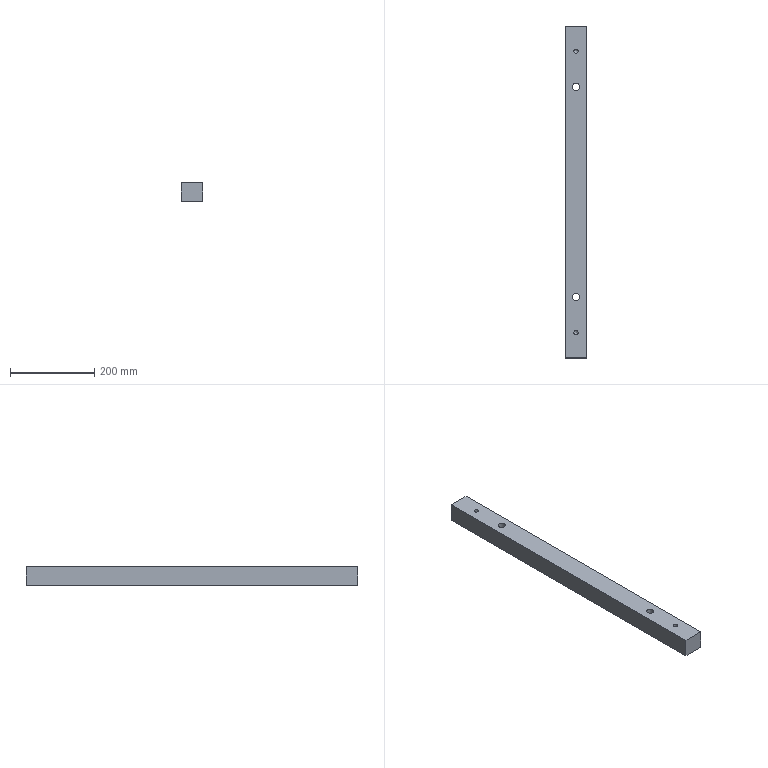Part | STEP file | 014_id2198_x_t | 1 solid | 16 faces | box 50 x 790 x 45 mm | volume 1744458 mm3 | plane 6 | cylinder 6 | cone 4 | commonest cylinder face diameters 10.3 x2 14 x2 17 x2
STEP:
#1=CARTESIAN_POINT('',(0.,0.,0.));
#2=DIRECTION('',(0.,0.,1.));
#3=DIRECTION('',(1.,0.,0.));
#4=AXIS2_PLACEMENT_3D('',#1,#2,#3);
#5=CARTESIAN_POINT('',(-521.65,-335.,230.));
#6=VERTEX_POINT('',#5);
#7=CARTESIAN_POINT('',(-516.5,-335.,230.));
#8=DIRECTION('',(0.,0.,-1.));
#9=DIRECTION('',(-1.,0.,0.));
#10=AXIS2_PLACEMENT_3D('',#7,#8,#9);
#11=CIRCLE('',#10,5.15);
#12=CARTESIAN_POINT('',(-541.5,-250.,230.));
#13=DIRECTION('',(0.,0.,-1.));
#14=DIRECTION('',(0.,-1.,0.));
#15=AXIS2_PLACEMENT_3D('',#12,#13,#14);
#16=PLANE('',#15);
#17=CARTESIAN_POINT('',(85.,-25.));
#18=DIRECTION('',(0.,1.));
#19=AXIS2_PLACEMENT_2D('',#17,#18);
#20=CIRCLE('',#19,5.15);
#21=(GEOMETRIC_REPRESENTATION_CONTEXT(2)PARAMETRIC_REPRESENTATION_CONTEXT()REPRESENTATION_CONTEXT('',''));
#22=DEFINITIONAL_REPRESENTATION('',(#20),#21);
#23=PCURVE('',#16,#22);
#24=CARTESIAN_POINT('',(-516.5,-335.,259.));
#25=DIRECTION('',(0.,0.,-1.));
#26=DIRECTION('',(-1.,0.,0.));
#27=AXIS2_PLACEMENT_3D('',#24,#25,#26);
#28=CYLINDRICAL_SURFACE('',#27,5.15);
#29=CARTESIAN_POINT('',(0.,29.));
#30=DIRECTION('',(1.,0.));
#31=VECTOR('',#30,1.);
#32=LINE('',#29,#31);
#33=(GEOMETRIC_REPRESENTATION_CONTEXT(2)PARAMETRIC_REPRESENTATION_CONTEXT()REPRESENTATION_CONTEXT('',''));
#34=DEFINITIONAL_REPRESENTATION('',(#32),#33);
#35=PCURVE('',#28,#34);
#36=SURFACE_CURVE('',#11,(#23,#35),.PCURVE_S1.);
#37=EDGE_CURVE('',#6,#6,#36,.T.);
#38=ORIENTED_EDGE('',*,*,#37,.T.);
#39=EDGE_LOOP('',(#38));
#40=FACE_BOUND('',#39,.T.);
#41=CARTESIAN_POINT('',(-521.65,335.,230.));
#42=VERTEX_POINT('',#41);
#43=CARTESIAN_POINT('',(-516.5,335.,230.));
#44=DIRECTION('',(0.,0.,1.));
#45=DIRECTION('',(-1.,0.,0.));
#46=AXIS2_PLACEMENT_3D('',#43,#44,#45);
#47=CIRCLE('',#46,5.15);
#48=CARTESIAN_POINT('',(-585.,-19.85));
#49=CARTESIAN_POINT('',(-576.08,-19.85));
#50=CARTESIAN_POINT('',(-580.54,-27.575));
#51=CARTESIAN_POINT('',(-585.,-35.3));
#52=CARTESIAN_POINT('',(-589.46,-27.575));
#53=CARTESIAN_POINT('',(-593.92,-19.85));
#54=CARTESIAN_POINT('',(-585.,-19.85));
#55=(BOUNDED_CURVE()B_SPLINE_CURVE(2,(#48,#49,#50,#51,#52,#53,#54),.UNSPECIFIED.,.T.,.F.)B_SPLINE_CURVE_WITH_KNOTS((1,2,2,2,2,1),(-2.094,0.,2.094,4.189,6.283,8.378),.UNSPECIFIED.)CURVE()GEOMETRIC_REPRESENTATION_ITEM()RATIONAL_B_SPLINE_CURVE((1.,0.5,1.,0.5,1.,0.5,1.))REPRESENTATION_ITEM(''));
#56=(GEOMETRIC_REPRESENTATION_CONTEXT(2)PARAMETRIC_REPRESENTATION_CONTEXT()REPRESENTATION_CONTEXT('',''));
#57=DEFINITIONAL_REPRESENTATION('',(#55),#56);
#58=PCURVE('',#16,#57);
#59=CARTESIAN_POINT('',(-516.5,335.,259.));
#60=DIRECTION('',(0.,0.,-1.));
#61=DIRECTION('',(-1.,0.,0.));
#62=AXIS2_PLACEMENT_3D('',#59,#60,#61);
#63=CYLINDRICAL_SURFACE('',#62,5.15);
#64=CARTESIAN_POINT('',(6.283,29.));
#65=DIRECTION('',(-1.,0.));
#66=VECTOR('',#65,1.);
#67=LINE('',#64,#66);
#68=(GEOMETRIC_REPRESENTATION_CONTEXT(2)PARAMETRIC_REPRESENTATION_CONTEXT()REPRESENTATION_CONTEXT('',''));
#69=DEFINITIONAL_REPRESENTATION('',(#67),#68);
#70=PCURVE('',#63,#69);
#71=SURFACE_CURVE('',#47,(#58,#70),.PCURVE_S1.);
#72=EDGE_CURVE('',#42,#42,#71,.T.);
#73=ORIENTED_EDGE('',*,*,#72,.F.);
#74=EDGE_LOOP('',(#73));
#75=FACE_BOUND('',#74,.T.);
#76=CARTESIAN_POINT('',(-541.5,-395.,230.));
#77=VERTEX_POINT('',#76);
#78=CARTESIAN_POINT('',(-491.5,-395.,230.));
#79=VERTEX_POINT('',#78);
#80=CARTESIAN_POINT('',(-541.5,-395.,230.));
#81=DIRECTION('',(1.,0.,0.));
#82=VECTOR('',#81,1.);
#83=LINE('',#80,#82);
#84=CARTESIAN_POINT('',(145.,0.));
#85=DIRECTION('',(0.,-1.));
#86=VECTOR('',#85,1.);
#87=LINE('',#84,#86);
#88=(GEOMETRIC_REPRESENTATION_CONTEXT(2)PARAMETRIC_REPRESENTATION_CONTEXT()REPRESENTATION_CONTEXT('',''));
#89=DEFINITIONAL_REPRESENTATION('',(#87),#88);
#90=PCURVE('',#16,#89);
#91=CARTESIAN_POINT('',(-541.5,-395.,-28.5));
#92=DIRECTION('',(0.,1.,0.));
#93=DIRECTION('',(0.,0.,-1.));
#94=AXIS2_PLACEMENT_3D('',#91,#92,#93);
#95=PLANE('',#94);
#96=CARTESIAN_POINT('',(-258.5,0.));
#97=DIRECTION('',(0.,-1.));
#98=VECTOR('',#97,1.);
#99=LINE('',#96,#98);
#100=(GEOMETRIC_REPRESENTATION_CONTEXT(2)PARAMETRIC_REPRESENTATION_CONTEXT()REPRESENTATION_CONTEXT('',''));
#101=DEFINITIONAL_REPRESENTATION('',(#99),#100);
#102=PCURVE('',#95,#101);
#103=SURFACE_CURVE('',#83,(#90,#102),.PCURVE_S1.);
#104=EDGE_CURVE('',#77,#79,#103,.T.);
#105=ORIENTED_EDGE('',*,*,#104,.T.);
#106=CARTESIAN_POINT('',(-491.5,395.,230.));
#107=VERTEX_POINT('',#106);
#108=CARTESIAN_POINT('',(-491.5,-250.,230.));
#109=DIRECTION('',(0.,-1.,0.));
#110=VECTOR('',#109,1.);
#111=LINE('',#108,#110);
#112=CARTESIAN_POINT('',(0.,-50.));
#113=DIRECTION('',(1.,0.));
#114=VECTOR('',#113,1.);
#115=LINE('',#112,#114);
#116=(GEOMETRIC_REPRESENTATION_CONTEXT(2)PARAMETRIC_REPRESENTATION_CONTEXT()REPRESENTATION_CONTEXT('',''));
#117=DEFINITIONAL_REPRESENTATION('',(#115),#116);
#118=PCURVE('',#16,#117);
#119=CARTESIAN_POINT('',(-491.5,-250.,-28.5));
#120=DIRECTION('',(-1.,0.,0.));
#121=DIRECTION('',(0.,0.,1.));
#122=AXIS2_PLACEMENT_3D('',#119,#120,#121);
#123=PLANE('',#122);
#124=CARTESIAN_POINT('',(258.5,0.));
#125=DIRECTION('',(0.,-1.));
#126=VECTOR('',#125,1.);
#127=LINE('',#124,#126);
#128=(GEOMETRIC_REPRESENTATION_CONTEXT(2)PARAMETRIC_REPRESENTATION_CONTEXT()REPRESENTATION_CONTEXT('',''));
#129=DEFINITIONAL_REPRESENTATION('',(#127),#128);
#130=PCURVE('',#123,#129);
#131=SURFACE_CURVE('',#111,(#118,#130),.PCURVE_S1.);
#132=EDGE_CURVE('',#107,#79,#131,.T.);
#133=ORIENTED_EDGE('',*,*,#132,.F.);
#134=CARTESIAN_POINT('',(-541.5,395.,230.));
#135=VERTEX_POINT('',#134);
#136=CARTESIAN_POINT('',(-541.5,395.,230.));
#137=DIRECTION('',(1.,0.,0.));
#138=VECTOR('',#137,1.);
#139=LINE('',#136,#138);
#140=CARTESIAN_POINT('',(-645.,0.));
#141=DIRECTION('',(0.,-1.));
#142=VECTOR('',#141,1.);
#143=LINE('',#140,#142);
#144=(GEOMETRIC_REPRESENTATION_CONTEXT(2)PARAMETRIC_REPRESENTATION_CONTEXT()REPRESENTATION_CONTEXT('',''));
#145=DEFINITIONAL_REPRESENTATION('',(#143),#144);
#146=PCURVE('',#16,#145);
#147=CARTESIAN_POINT('',(-541.5,395.,-28.5));
#148=DIRECTION('',(0.,1.,0.));
#149=DIRECTION('',(0.,0.,-1.));
#150=AXIS2_PLACEMENT_3D('',#147,#148,#149);
#151=PLANE('',#150);
#152=CARTESIAN_POINT('',(-258.5,0.));
#153=DIRECTION('',(0.,-1.));
#154=VECTOR('',#153,1.);
#155=LINE('',#152,#154);
#156=(GEOMETRIC_REPRESENTATION_CONTEXT(2)PARAMETRIC_REPRESENTATION_CONTEXT()REPRESENTATION_CONTEXT('',''));
#157=DEFINITIONAL_REPRESENTATION('',(#155),#156);
#158=PCURVE('',#151,#157);
#159=SURFACE_CURVE('',#139,(#146,#158),.PCURVE_S1.);
#160=EDGE_CURVE('',#135,#107,#159,.T.);
#161=ORIENTED_EDGE('',*,*,#160,.F.);
#162=CARTESIAN_POINT('',(-541.5,-250.,230.));
#163=DIRECTION('',(0.,-1.,0.));
#164=VECTOR('',#163,1.);
#165=LINE('',#162,#164);
#166=CARTESIAN_POINT('',(0.,0.));
#167=DIRECTION('',(1.,0.));
#168=VECTOR('',#167,1.);
#169=LINE('',#166,#168);
#170=(GEOMETRIC_REPRESENTATION_CONTEXT(2)PARAMETRIC_REPRESENTATION_CONTEXT()REPRESENTATION_CONTEXT('',''));
#171=DEFINITIONAL_REPRESENTATION('',(#169),#170);
#172=PCURVE('',#16,#171);
#173=CARTESIAN_POINT('',(-541.5,-250.,-28.5));
#174=DIRECTION('',(-1.,0.,0.));
#175=DIRECTION('',(0.,0.,1.));
#176=AXIS2_PLACEMENT_3D('',#173,#174,#175);
#177=PLANE('',#176);
#178=CARTESIAN_POINT('',(258.5,0.));
#179=DIRECTION('',(0.,-1.));
#180=VECTOR('',#179,1.);
#181=LINE('',#178,#180);
#182=(GEOMETRIC_REPRESENTATION_CONTEXT(2)PARAMETRIC_REPRESENTATION_CONTEXT()REPRESENTATION_CONTEXT('',''));
#183=DEFINITIONAL_REPRESENTATION('',(#181),#182);
#184=PCURVE('',#177,#183);
#185=SURFACE_CURVE('',#165,(#172,#184),.PCURVE_S1.);
#186=EDGE_CURVE('',#135,#77,#185,.T.);
#187=ORIENTED_EDGE('',*,*,#186,.T.);
#188=EDGE_LOOP('',(#105,#133,#161,#187));
#189=FACE_BOUND('',#188,.T.);
#190=CARTESIAN_POINT('',(-525.,250.,230.));
#191=VERTEX_POINT('',#190);
#192=CARTESIAN_POINT('',(-516.5,250.,230.));
#193=DIRECTION('',(0.,0.,-1.));
#194=DIRECTION('',(-1.,0.,0.));
#195=AXIS2_PLACEMENT_3D('',#192,#193,#194);
#196=CIRCLE('',#195,8.5);
#197=CARTESIAN_POINT('',(-500.,-25.));
#198=DIRECTION('',(0.,1.));
#199=AXIS2_PLACEMENT_2D('',#197,#198);
#200=CIRCLE('',#199,8.5);
#201=(GEOMETRIC_REPRESENTATION_CONTEXT(2)PARAMETRIC_REPRESENTATION_CONTEXT()REPRESENTATION_CONTEXT('',''));
#202=DEFINITIONAL_REPRESENTATION('',(#200),#201);
#203=PCURVE('',#16,#202);
#204=CARTESIAN_POINT('',(-516.5,250.,150.016));
#205=DIRECTION('',(0.,0.,1.));
#206=DIRECTION('',(1.,0.,0.));
#207=AXIS2_PLACEMENT_3D('',#204,#205,#206);
#208=CYLINDRICAL_SURFACE('',#207,8.5);
#209=CARTESIAN_POINT('',(9.425,79.984));
#210=DIRECTION('',(-1.,0.));
#211=VECTOR('',#210,1.);
#212=LINE('',#209,#211);
#213=(GEOMETRIC_REPRESENTATION_CONTEXT(2)PARAMETRIC_REPRESENTATION_CONTEXT()REPRESENTATION_CONTEXT('',''));
#214=DEFINITIONAL_REPRESENTATION('',(#212),#213);
#215=PCURVE('',#208,#214);
#216=SURFACE_CURVE('',#196,(#203,#215),.PCURVE_S1.);
#217=EDGE_CURVE('',#191,#191,#216,.T.);
#218=ORIENTED_EDGE('',*,*,#217,.T.);
#219=EDGE_LOOP('',(#218));
#220=FACE_BOUND('',#219,.T.);
#221=CARTESIAN_POINT('',(-525.,-250.,230.));
#222=VERTEX_POINT('',#221);
#223=CARTESIAN_POINT('',(-516.5,-250.,230.));
#224=DIRECTION('',(0.,0.,-1.));
#225=DIRECTION('',(-1.,0.,0.));
#226=AXIS2_PLACEMENT_3D('',#223,#224,#225);
#227=CIRCLE('',#226,8.5);
#228=CARTESIAN_POINT('',(0.,-25.));
#229=DIRECTION('',(0.,1.));
#230=AXIS2_PLACEMENT_2D('',#228,#229);
#231=CIRCLE('',#230,8.5);
#232=(GEOMETRIC_REPRESENTATION_CONTEXT(2)PARAMETRIC_REPRESENTATION_CONTEXT()REPRESENTATION_CONTEXT('',''));
#233=DEFINITIONAL_REPRESENTATION('',(#231),#232);
#234=PCURVE('',#16,#233);
#235=CARTESIAN_POINT('',(-516.5,-250.,150.016));
#236=DIRECTION('',(0.,0.,1.));
#237=DIRECTION('',(1.,0.,0.));
#238=AXIS2_PLACEMENT_3D('',#235,#236,#237);
#239=CYLINDRICAL_SURFACE('',#238,8.5);
#240=CARTESIAN_POINT('',(9.425,79.984));
#241=DIRECTION('',(-1.,0.));
#242=VECTOR('',#241,1.);
#243=LINE('',#240,#242);
#244=(GEOMETRIC_REPRESENTATION_CONTEXT(2)PARAMETRIC_REPRESENTATION_CONTEXT()REPRESENTATION_CONTEXT('',''));
#245=DEFINITIONAL_REPRESENTATION('',(#243),#244);
#246=PCURVE('',#239,#245);
#247=SURFACE_CURVE('',#227,(#234,#246),.PCURVE_S1.);
#248=EDGE_CURVE('',#222,#222,#247,.T.);
#249=ORIENTED_EDGE('',*,*,#248,.T.);
#250=EDGE_LOOP('',(#249));
#251=FACE_BOUND('',#250,.T.);
#252=ADVANCED_FACE('',(#40,#75,#189,#220,#251),#16,.F.);
#253=CARTESIAN_POINT('',(-525.,-250.,185.));
#254=VERTEX_POINT('',#253);
#255=CARTESIAN_POINT('',(-516.5,-250.,185.));
#256=DIRECTION('',(0.,0.,-1.));
#257=DIRECTION('',(-1.,0.,0.));
#258=AXIS2_PLACEMENT_3D('',#255,#256,#257);
#259=CIRCLE('',#258,8.5);
#260=CARTESIAN_POINT('',(-336.5,-40.,185.));
#261=DIRECTION('',(0.,0.,-1.));
#262=DIRECTION('',(1.,0.,0.));
#263=AXIS2_PLACEMENT_3D('',#260,#261,#262);
#264=PLANE('',#263);
#265=CARTESIAN_POINT('',(-180.,210.));
#266=DIRECTION('',(-1.,0.));
#267=AXIS2_PLACEMENT_2D('',#265,#266);
#268=CIRCLE('',#267,8.5);
#269=(GEOMETRIC_REPRESENTATION_CONTEXT(2)PARAMETRIC_REPRESENTATION_CONTEXT()REPRESENTATION_CONTEXT('',''));
#270=DEFINITIONAL_REPRESENTATION('',(#268),#269);
#271=PCURVE('',#264,#270);
#272=CARTESIAN_POINT('',(9.425,34.984));
#273=DIRECTION('',(-1.,0.));
#274=VECTOR('',#273,1.);
#275=LINE('',#272,#274);
#276=(GEOMETRIC_REPRESENTATION_CONTEXT(2)PARAMETRIC_REPRESENTATION_CONTEXT()REPRESENTATION_CONTEXT('',''));
#277=DEFINITIONAL_REPRESENTATION('',(#275),#276);
#278=PCURVE('',#239,#277);
#279=SURFACE_CURVE('',#259,(#271,#278),.PCURVE_S1.);
#280=EDGE_CURVE('',#254,#254,#279,.T.);
#281=ORIENTED_EDGE('',*,*,#280,.F.);
#282=EDGE_LOOP('',(#281));
#283=FACE_BOUND('',#282,.T.);
#284=CARTESIAN_POINT('',(-525.,250.,185.));
#285=VERTEX_POINT('',#284);
#286=CARTESIAN_POINT('',(-516.5,250.,185.));
#287=DIRECTION('',(0.,0.,-1.));
#288=DIRECTION('',(-1.,0.,0.));
#289=AXIS2_PLACEMENT_3D('',#286,#287,#288);
#290=CIRCLE('',#289,8.5);
#291=CARTESIAN_POINT('',(-180.,-290.));
#292=DIRECTION('',(-1.,0.));
#293=AXIS2_PLACEMENT_2D('',#291,#292);
#294=CIRCLE('',#293,8.5);
#295=(GEOMETRIC_REPRESENTATION_CONTEXT(2)PARAMETRIC_REPRESENTATION_CONTEXT()REPRESENTATION_CONTEXT('',''));
#296=DEFINITIONAL_REPRESENTATION('',(#294),#295);
#297=PCURVE('',#264,#296);
#298=CARTESIAN_POINT('',(9.425,34.984));
#299=DIRECTION('',(-1.,0.));
#300=VECTOR('',#299,1.);
#301=LINE('',#298,#300);
#302=(GEOMETRIC_REPRESENTATION_CONTEXT(2)PARAMETRIC_REPRESENTATION_CONTEXT()REPRESENTATION_CONTEXT('',''));
#303=DEFINITIONAL_REPRESENTATION('',(#301),#302);
#304=PCURVE('',#208,#303);
#305=SURFACE_CURVE('',#290,(#297,#304),.PCURVE_S1.);
#306=EDGE_CURVE('',#285,#285,#305,.T.);
#307=ORIENTED_EDGE('',*,*,#306,.F.);
#308=EDGE_LOOP('',(#307));
#309=FACE_BOUND('',#308,.T.);
#310=CARTESIAN_POINT('',(-523.5,-370.,185.));
#311=VERTEX_POINT('',#310);
#312=CARTESIAN_POINT('',(-516.5,-370.,185.));
#313=DIRECTION('',(0.,0.,-1.));
#314=DIRECTION('',(-1.,0.,0.));
#315=AXIS2_PLACEMENT_3D('',#312,#313,#314);
#316=CIRCLE('',#315,7.);
#317=CARTESIAN_POINT('',(-180.,330.));
#318=DIRECTION('',(-1.,0.));
#319=AXIS2_PLACEMENT_2D('',#317,#318);
#320=CIRCLE('',#319,7.);
#321=(GEOMETRIC_REPRESENTATION_CONTEXT(2)PARAMETRIC_REPRESENTATION_CONTEXT()REPRESENTATION_CONTEXT('',''));
#322=DEFINITIONAL_REPRESENTATION('',(#320),#321);
#323=PCURVE('',#264,#322);
#324=CARTESIAN_POINT('',(-516.5,-370.,121.));
#325=DIRECTION('',(0.,0.,1.));
#326=DIRECTION('',(1.,0.,0.));
#327=AXIS2_PLACEMENT_3D('',#324,#325,#326);
#328=CYLINDRICAL_SURFACE('',#327,7.);
#329=CARTESIAN_POINT('',(9.425,64.));
#330=DIRECTION('',(-1.,0.));
#331=VECTOR('',#330,1.);
#332=LINE('',#329,#331);
#333=(GEOMETRIC_REPRESENTATION_CONTEXT(2)PARAMETRIC_REPRESENTATION_CONTEXT()REPRESENTATION_CONTEXT('',''));
#334=DEFINITIONAL_REPRESENTATION('',(#332),#333);
#335=PCURVE('',#328,#334);
#336=SURFACE_CURVE('',#316,(#323,#335),.PCURVE_S1.);
#337=EDGE_CURVE('',#311,#311,#336,.T.);
#338=ORIENTED_EDGE('',*,*,#337,.F.);
#339=EDGE_LOOP('',(#338));
#340=FACE_BOUND('',#339,.T.);
#341=CARTESIAN_POINT('',(-523.5,370.,185.));
#342=VERTEX_POINT('',#341);
#343=CARTESIAN_POINT('',(-509.5,370.,185.));
#344=VERTEX_POINT('',#343);
#345=CARTESIAN_POINT('',(-516.5,370.,185.));
#346=DIRECTION('',(0.,0.,-1.));
#347=DIRECTION('',(-1.,0.,0.));
#348=AXIS2_PLACEMENT_3D('',#345,#346,#347);
#349=CIRCLE('',#348,7.);
#350=CARTESIAN_POINT('',(-180.,-410.));
#351=DIRECTION('',(-1.,0.));
#352=AXIS2_PLACEMENT_2D('',#350,#351);
#353=CIRCLE('',#352,7.);
#354=(GEOMETRIC_REPRESENTATION_CONTEXT(2)PARAMETRIC_REPRESENTATION_CONTEXT()REPRESENTATION_CONTEXT('',''));
#355=DEFINITIONAL_REPRESENTATION('',(#353),#354);
#356=PCURVE('',#264,#355);
#357=CARTESIAN_POINT('',(-516.5,370.,121.));
#358=DIRECTION('',(0.,0.,1.));
#359=DIRECTION('',(1.,0.,0.));
#360=AXIS2_PLACEMENT_3D('',#357,#358,#359);
#361=CYLINDRICAL_SURFACE('',#360,7.);
#362=CARTESIAN_POINT('',(3.142,64.));
#363=DIRECTION('',(-1.,0.));
#364=VECTOR('',#363,1.);
#365=LINE('',#362,#364);
#366=(GEOMETRIC_REPRESENTATION_CONTEXT(2)PARAMETRIC_REPRESENTATION_CONTEXT()REPRESENTATION_CONTEXT('',''));
#367=DEFINITIONAL_REPRESENTATION('',(#365),#366);
#368=PCURVE('',#361,#367);
#369=SURFACE_CURVE('',#349,(#356,#368),.PCURVE_S1.);
#370=EDGE_CURVE('',#342,#344,#369,.T.);
#371=ORIENTED_EDGE('',*,*,#370,.F.);
#372=CARTESIAN_POINT('',(-516.5,370.,185.));
#373=DIRECTION('',(0.,0.,-1.));
#374=DIRECTION('',(-1.,0.,0.));
#375=AXIS2_PLACEMENT_3D('',#372,#373,#374);
#376=CIRCLE('',#375,7.);
#377=CARTESIAN_POINT('',(-180.,-410.));
#378=DIRECTION('',(-1.,0.));
#379=AXIS2_PLACEMENT_2D('',#377,#378);
#380=CIRCLE('',#379,7.);
#381=(GEOMETRIC_REPRESENTATION_CONTEXT(2)PARAMETRIC_REPRESENTATION_CONTEXT()REPRESENTATION_CONTEXT('',''));
#382=DEFINITIONAL_REPRESENTATION('',(#380),#381);
#383=PCURVE('',#264,#382);
#384=CARTESIAN_POINT('',(9.425,64.));
#385=DIRECTION('',(-1.,0.));
#386=VECTOR('',#385,1.);
#387=LINE('',#384,#386);
#388=(GEOMETRIC_REPRESENTATION_CONTEXT(2)PARAMETRIC_REPRESENTATION_CONTEXT()REPRESENTATION_CONTEXT('',''));
#389=DEFINITIONAL_REPRESENTATION('',(#387),#388);
#390=PCURVE('',#361,#389);
#391=SURFACE_CURVE('',#376,(#383,#390),.PCURVE_S1.);
#392=EDGE_CURVE('',#344,#342,#391,.T.);
#393=ORIENTED_EDGE('',*,*,#392,.F.);
#394=EDGE_LOOP('',(#371,#393));
#395=FACE_BOUND('',#394,.T.);
#396=CARTESIAN_POINT('',(-541.5,395.,185.));
#397=VERTEX_POINT('',#396);
#398=CARTESIAN_POINT('',(-491.5,395.,185.));
#399=VERTEX_POINT('',#398);
#400=CARTESIAN_POINT('',(-336.5,395.,185.));
#401=DIRECTION('',(1.,0.,0.));
#402=VECTOR('',#401,1.);
#403=LINE('',#400,#402);
#404=CARTESIAN_POINT('',(0.,-435.));
#405=DIRECTION('',(1.,0.));
#406=VECTOR('',#405,1.);
#407=LINE('',#404,#406);
#408=(GEOMETRIC_REPRESENTATION_CONTEXT(2)PARAMETRIC_REPRESENTATION_CONTEXT()REPRESENTATION_CONTEXT('',''));
#409=DEFINITIONAL_REPRESENTATION('',(#407),#408);
#410=PCURVE('',#264,#409);
#411=CARTESIAN_POINT('',(-213.5,-205.));
#412=DIRECTION('',(0.,-1.));
#413=VECTOR('',#412,1.);
#414=LINE('',#411,#413);
#415=(GEOMETRIC_REPRESENTATION_CONTEXT(2)PARAMETRIC_REPRESENTATION_CONTEXT()REPRESENTATION_CONTEXT('',''));
#416=DEFINITIONAL_REPRESENTATION('',(#414),#415);
#417=PCURVE('',#151,#416);
#418=SURFACE_CURVE('',#403,(#410,#417),.PCURVE_S1.);
#419=EDGE_CURVE('',#397,#399,#418,.T.);
#420=ORIENTED_EDGE('',*,*,#419,.T.);
#421=CARTESIAN_POINT('',(-491.5,-395.,185.));
#422=VERTEX_POINT('',#421);
#423=CARTESIAN_POINT('',(-491.5,-250.,185.));
#424=DIRECTION('',(0.,-1.,0.));
#425=VECTOR('',#424,1.);
#426=LINE('',#423,#425);
#427=CARTESIAN_POINT('',(-155.,210.));
#428=DIRECTION('',(0.,1.));
#429=VECTOR('',#428,1.);
#430=LINE('',#427,#429);
#431=(GEOMETRIC_REPRESENTATION_CONTEXT(2)PARAMETRIC_REPRESENTATION_CONTEXT()REPRESENTATION_CONTEXT('',''));
#432=DEFINITIONAL_REPRESENTATION('',(#430),#431);
#433=PCURVE('',#264,#432);
#434=CARTESIAN_POINT('',(213.5,0.));
#435=DIRECTION('',(0.,-1.));
#436=VECTOR('',#435,1.);
#437=LINE('',#434,#436);
#438=(GEOMETRIC_REPRESENTATION_CONTEXT(2)PARAMETRIC_REPRESENTATION_CONTEXT()REPRESENTATION_CONTEXT('',''));
#439=DEFINITIONAL_REPRESENTATION('',(#437),#438);
#440=PCURVE('',#123,#439);
#441=SURFACE_CURVE('',#426,(#433,#440),.PCURVE_S1.);
#442=EDGE_CURVE('',#399,#422,#441,.T.);
#443=ORIENTED_EDGE('',*,*,#442,.T.);
#444=CARTESIAN_POINT('',(-541.5,-395.,185.));
#445=VERTEX_POINT('',#444);
#446=CARTESIAN_POINT('',(-336.5,-395.,185.));
#447=DIRECTION('',(1.,0.,0.));
#448=VECTOR('',#447,1.);
#449=LINE('',#446,#448);
#450=CARTESIAN_POINT('',(0.,355.));
#451=DIRECTION('',(1.,0.));
#452=VECTOR('',#451,1.);
#453=LINE('',#450,#452);
#454=(GEOMETRIC_REPRESENTATION_CONTEXT(2)PARAMETRIC_REPRESENTATION_CONTEXT()REPRESENTATION_CONTEXT('',''));
#455=DEFINITIONAL_REPRESENTATION('',(#453),#454);
#456=PCURVE('',#264,#455);
#457=CARTESIAN_POINT('',(-213.5,-205.));
#458=DIRECTION('',(0.,-1.));
#459=VECTOR('',#458,1.);
#460=LINE('',#457,#459);
#461=(GEOMETRIC_REPRESENTATION_CONTEXT(2)PARAMETRIC_REPRESENTATION_CONTEXT()REPRESENTATION_CONTEXT('',''));
#462=DEFINITIONAL_REPRESENTATION('',(#460),#461);
#463=PCURVE('',#95,#462);
#464=SURFACE_CURVE('',#449,(#456,#463),.PCURVE_S1.);
#465=EDGE_CURVE('',#445,#422,#464,.T.);
#466=ORIENTED_EDGE('',*,*,#465,.F.);
#467=CARTESIAN_POINT('',(-541.5,-40.,185.));
#468=DIRECTION('',(0.,1.,0.));
#469=VECTOR('',#468,1.);
#470=LINE('',#467,#469);
#471=CARTESIAN_POINT('',(-205.,0.));
#472=DIRECTION('',(0.,-1.));
#473=VECTOR('',#472,1.);
#474=LINE('',#471,#473);
#475=(GEOMETRIC_REPRESENTATION_CONTEXT(2)PARAMETRIC_REPRESENTATION_CONTEXT()REPRESENTATION_CONTEXT('',''));
#476=DEFINITIONAL_REPRESENTATION('',(#474),#475);
#477=PCURVE('',#264,#476);
#478=CARTESIAN_POINT('',(213.5,210.));
#479=DIRECTION('',(0.,1.));
#480=VECTOR('',#479,1.);
#481=LINE('',#478,#480);
#482=(GEOMETRIC_REPRESENTATION_CONTEXT(2)PARAMETRIC_REPRESENTATION_CONTEXT()REPRESENTATION_CONTEXT('',''));
#483=DEFINITIONAL_REPRESENTATION('',(#481),#482);
#484=PCURVE('',#177,#483);
#485=SURFACE_CURVE('',#470,(#477,#484),.PCURVE_S1.);
#486=EDGE_CURVE('',#445,#397,#485,.T.);
#487=ORIENTED_EDGE('',*,*,#486,.T.);
#488=EDGE_LOOP('',(#420,#443,#466,#487));
#489=FACE_BOUND('',#488,.T.);
#490=ADVANCED_FACE('',(#283,#309,#340,#395,#489),#264,.T.);
#491=ORIENTED_EDGE('',*,*,#442,.F.);
#492=CARTESIAN_POINT('',(-491.5,395.,-28.5));
#493=DIRECTION('',(0.,0.,1.));
#494=VECTOR('',#493,1.);
#495=LINE('',#492,#494);
#496=CARTESIAN_POINT('',(0.,645.));
#497=DIRECTION('',(1.,0.));
#498=VECTOR('',#497,1.);
#499=LINE('',#496,#498);
#500=(GEOMETRIC_REPRESENTATION_CONTEXT(2)PARAMETRIC_REPRESENTATION_CONTEXT()REPRESENTATION_CONTEXT('',''));
#501=DEFINITIONAL_REPRESENTATION('',(#499),#500);
#502=PCURVE('',#123,#501);
#503=CARTESIAN_POINT('',(0.,-50.));
#504=DIRECTION('',(-1.,0.));
#505=VECTOR('',#504,1.);
#506=LINE('',#503,#505);
#507=(GEOMETRIC_REPRESENTATION_CONTEXT(2)PARAMETRIC_REPRESENTATION_CONTEXT()REPRESENTATION_CONTEXT('',''));
#508=DEFINITIONAL_REPRESENTATION('',(#506),#507);
#509=PCURVE('',#151,#508);
#510=SURFACE_CURVE('',#495,(#502,#509),.PCURVE_S1.);
#511=EDGE_CURVE('',#399,#107,#510,.T.);
#512=ORIENTED_EDGE('',*,*,#511,.T.);
#513=ORIENTED_EDGE('',*,*,#132,.T.);
#514=CARTESIAN_POINT('',(-491.5,-395.,-28.5));
#515=DIRECTION('',(0.,0.,-1.));
#516=VECTOR('',#515,1.);
#517=LINE('',#514,#516);
#518=CARTESIAN_POINT('',(0.,-145.));
#519=DIRECTION('',(-1.,0.));
#520=VECTOR('',#519,1.);
#521=LINE('',#518,#520);
#522=(GEOMETRIC_REPRESENTATION_CONTEXT(2)PARAMETRIC_REPRESENTATION_CONTEXT()REPRESENTATION_CONTEXT('',''));
#523=DEFINITIONAL_REPRESENTATION('',(#521),#522);
#524=PCURVE('',#123,#523);
#525=CARTESIAN_POINT('',(0.,-50.));
#526=DIRECTION('',(1.,0.));
#527=VECTOR('',#526,1.);
#528=LINE('',#525,#527);
#529=(GEOMETRIC_REPRESENTATION_CONTEXT(2)PARAMETRIC_REPRESENTATION_CONTEXT()REPRESENTATION_CONTEXT('',''));
#530=DEFINITIONAL_REPRESENTATION('',(#528),#529);
#531=PCURVE('',#95,#530);
#532=SURFACE_CURVE('',#517,(#524,#531),.PCURVE_S1.);
#533=EDGE_CURVE('',#79,#422,#532,.T.);
#534=ORIENTED_EDGE('',*,*,#533,.T.);
#535=EDGE_LOOP('',(#491,#512,#513,#534));
#536=FACE_BOUND('',#535,.T.);
#537=ADVANCED_FACE('',(#536),#123,.F.);
#538=ORIENTED_EDGE('',*,*,#465,.T.);
#539=ORIENTED_EDGE('',*,*,#533,.F.);
#540=ORIENTED_EDGE('',*,*,#104,.F.);
#541=CARTESIAN_POINT('',(-541.5,-395.,-28.5));
#542=DIRECTION('',(0.,0.,-1.));
#543=VECTOR('',#542,1.);
#544=LINE('',#541,#543);
#545=CARTESIAN_POINT('',(0.,0.));
#546=DIRECTION('',(1.,0.));
#547=VECTOR('',#546,1.);
#548=LINE('',#545,#547);
#549=(GEOMETRIC_REPRESENTATION_CONTEXT(2)PARAMETRIC_REPRESENTATION_CONTEXT()REPRESENTATION_CONTEXT('',''));
#550=DEFINITIONAL_REPRESENTATION('',(#548),#549);
#551=PCURVE('',#95,#550);
#552=CARTESIAN_POINT('',(0.,-145.));
#553=DIRECTION('',(-1.,0.));
#554=VECTOR('',#553,1.);
#555=LINE('',#552,#554);
#556=(GEOMETRIC_REPRESENTATION_CONTEXT(2)PARAMETRIC_REPRESENTATION_CONTEXT()REPRESENTATION_CONTEXT('',''));
#557=DEFINITIONAL_REPRESENTATION('',(#555),#556);
#558=PCURVE('',#177,#557);
#559=SURFACE_CURVE('',#544,(#551,#558),.PCURVE_S1.);
#560=EDGE_CURVE('',#77,#445,#559,.T.);
#561=ORIENTED_EDGE('',*,*,#560,.T.);
#562=EDGE_LOOP('',(#538,#539,#540,#561));
#563=FACE_BOUND('',#562,.T.);
#564=ADVANCED_FACE('',(#563),#95,.F.);
#565=CARTESIAN_POINT('',(-541.5,395.,-28.5));
#566=DIRECTION('',(0.,0.,1.));
#567=VECTOR('',#566,1.);
#568=LINE('',#565,#567);
#569=CARTESIAN_POINT('',(0.,645.));
#570=DIRECTION('',(1.,0.));
#571=VECTOR('',#570,1.);
#572=LINE('',#569,#571);
#573=(GEOMETRIC_REPRESENTATION_CONTEXT(2)PARAMETRIC_REPRESENTATION_CONTEXT()REPRESENTATION_CONTEXT('',''));
#574=DEFINITIONAL_REPRESENTATION('',(#572),#573);
#575=PCURVE('',#177,#574);
#576=CARTESIAN_POINT('',(0.,0.));
#577=DIRECTION('',(-1.,0.));
#578=VECTOR('',#577,1.);
#579=LINE('',#576,#578);
#580=(GEOMETRIC_REPRESENTATION_CONTEXT(2)PARAMETRIC_REPRESENTATION_CONTEXT()REPRESENTATION_CONTEXT('',''));
#581=DEFINITIONAL_REPRESENTATION('',(#579),#580);
#582=PCURVE('',#151,#581);
#583=SURFACE_CURVE('',#568,(#575,#582),.PCURVE_S1.);
#584=EDGE_CURVE('',#397,#135,#583,.T.);
#585=ORIENTED_EDGE('',*,*,#584,.F.);
#586=ORIENTED_EDGE('',*,*,#486,.F.);
#587=ORIENTED_EDGE('',*,*,#560,.F.);
#588=ORIENTED_EDGE('',*,*,#186,.F.);
#589=EDGE_LOOP('',(#585,#586,#587,#588));
#590=FACE_BOUND('',#589,.T.);
#591=ADVANCED_FACE('',(#590),#177,.T.);
#592=ORIENTED_EDGE('',*,*,#511,.F.);
#593=ORIENTED_EDGE('',*,*,#419,.F.);
#594=ORIENTED_EDGE('',*,*,#584,.T.);
#595=ORIENTED_EDGE('',*,*,#160,.T.);
#596=EDGE_LOOP('',(#592,#593,#594,#595));
#597=FACE_BOUND('',#596,.T.);
#598=ADVANCED_FACE('',(#597),#151,.T.);
#599=ORIENTED_EDGE('',*,*,#392,.F.);
#600=CARTESIAN_POINT('',(-509.5,370.,209.459));
#601=VERTEX_POINT('',#600);
#602=CARTESIAN_POINT('',(-509.5,370.,185.));
#603=CARTESIAN_POINT('',(-509.5,370.,209.459));
#604=B_SPLINE_CURVE_WITH_KNOTS('',1,(#602,#603),.UNSPECIFIED.,.F.,.F.,(2,2),(64.,88.459),.PIECEWISE_BEZIER_KNOTS.);
#605=CARTESIAN_POINT('',(6.283,0.));
#606=DIRECTION('',(0.,1.));
#607=VECTOR('',#606,1.);
#608=LINE('',#605,#607);
#609=(GEOMETRIC_REPRESENTATION_CONTEXT(2)PARAMETRIC_REPRESENTATION_CONTEXT()REPRESENTATION_CONTEXT('',''));
#610=DEFINITIONAL_REPRESENTATION('',(#608),#609);
#611=PCURVE('',#361,#610);
#612=CARTESIAN_POINT('',(0.,0.));
#613=DIRECTION('',(0.,1.));
#614=VECTOR('',#613,1.);
#615=LINE('',#612,#614);
#616=(GEOMETRIC_REPRESENTATION_CONTEXT(2)PARAMETRIC_REPRESENTATION_CONTEXT()REPRESENTATION_CONTEXT('',''));
#617=DEFINITIONAL_REPRESENTATION('',(#615),#616);
#618=PCURVE('',#361,#617);
#619=SEAM_CURVE('',#604,(#611,#618),.PCURVE_S1.);
#620=EDGE_CURVE('',#344,#601,#619,.T.);
#621=ORIENTED_EDGE('',*,*,#620,.T.);
#622=CARTESIAN_POINT('',(-523.5,370.,209.459));
#623=VERTEX_POINT('',#622);
#624=CARTESIAN_POINT('',(-516.5,370.,209.459));
#625=DIRECTION('',(0.,0.,-1.));
#626=DIRECTION('',(1.,0.,0.));
#627=AXIS2_PLACEMENT_3D('',#624,#625,#626);
#628=CIRCLE('',#627,7.);
#629=CARTESIAN_POINT('',(6.283,88.459));
#630=DIRECTION('',(-1.,0.));
#631=VECTOR('',#630,1.);
#632=LINE('',#629,#631);
#633=(GEOMETRIC_REPRESENTATION_CONTEXT(2)PARAMETRIC_REPRESENTATION_CONTEXT()REPRESENTATION_CONTEXT('',''));
#634=DEFINITIONAL_REPRESENTATION('',(#632),#633);
#635=PCURVE('',#361,#634);
#636=CARTESIAN_POINT('',(-516.5,370.,209.459));
#637=DIRECTION('',(0.,0.,-1.));
#638=DIRECTION('',(-1.,0.,0.));
#639=AXIS2_PLACEMENT_3D('',#636,#637,#638);
#640=CONICAL_SURFACE('',#639,7.,1.047);
#641=CARTESIAN_POINT('',(3.142,0.));
#642=DIRECTION('',(1.,0.));
#643=VECTOR('',#642,1.);
#644=LINE('',#641,#643);
#645=(GEOMETRIC_REPRESENTATION_CONTEXT(2)PARAMETRIC_REPRESENTATION_CONTEXT()REPRESENTATION_CONTEXT('',''));
#646=DEFINITIONAL_REPRESENTATION('',(#644),#645);
#647=PCURVE('',#640,#646);
#648=SURFACE_CURVE('',#628,(#635,#647),.PCURVE_S1.);
#649=EDGE_CURVE('',#601,#623,#648,.T.);
#650=ORIENTED_EDGE('',*,*,#649,.T.);
#651=CARTESIAN_POINT('',(-516.5,370.,209.459));
#652=DIRECTION('',(0.,0.,-1.));
#653=DIRECTION('',(1.,0.,0.));
#654=AXIS2_PLACEMENT_3D('',#651,#652,#653);
#655=CIRCLE('',#654,7.);
#656=CARTESIAN_POINT('',(6.283,88.459));
#657=DIRECTION('',(-1.,0.));
#658=VECTOR('',#657,1.);
#659=LINE('',#656,#658);
#660=(GEOMETRIC_REPRESENTATION_CONTEXT(2)PARAMETRIC_REPRESENTATION_CONTEXT()REPRESENTATION_CONTEXT('',''));
#661=DEFINITIONAL_REPRESENTATION('',(#659),#660);
#662=PCURVE('',#361,#661);
#663=CARTESIAN_POINT('',(-3.142,0.));
#664=DIRECTION('',(1.,0.));
#665=VECTOR('',#664,1.);
#666=LINE('',#663,#665);
#667=(GEOMETRIC_REPRESENTATION_CONTEXT(2)PARAMETRIC_REPRESENTATION_CONTEXT()REPRESENTATION_CONTEXT('',''));
#668=DEFINITIONAL_REPRESENTATION('',(#666),#667);
#669=PCURVE('',#640,#668);
#670=SURFACE_CURVE('',#655,(#662,#669),.PCURVE_S1.);
#671=EDGE_CURVE('',#623,#601,#670,.T.);
#672=ORIENTED_EDGE('',*,*,#671,.T.);
#673=ORIENTED_EDGE('',*,*,#620,.F.);
#674=ORIENTED_EDGE('',*,*,#370,.F.);
#675=EDGE_LOOP('',(#599,#621,#650,#672,#673,#674));
#676=FACE_BOUND('',#675,.F.);
#677=ADVANCED_FACE('',(#676),#361,.F.);
#678=CARTESIAN_POINT('',(-516.5,370.,213.5));
#679=VERTEX_POINT('',#678);
#680=CARTESIAN_POINT('',(-516.5,370.,213.5));
#681=CARTESIAN_POINT('',(-523.5,370.,209.459));
#682=B_SPLINE_CURVE_WITH_KNOTS('',1,(#680,#681),.UNSPECIFIED.,.F.,.F.,(2,2),(-8.083,0.),.PIECEWISE_BEZIER_KNOTS.);
#683=CARTESIAN_POINT('',(6.283,0.));
#684=DIRECTION('',(0.,1.));
#685=VECTOR('',#684,1.);
#686=LINE('',#683,#685);
#687=(GEOMETRIC_REPRESENTATION_CONTEXT(2)PARAMETRIC_REPRESENTATION_CONTEXT()REPRESENTATION_CONTEXT('',''));
#688=DEFINITIONAL_REPRESENTATION('',(#686),#687);
#689=PCURVE('',#640,#688);
#690=CARTESIAN_POINT('',(0.,0.));
#691=DIRECTION('',(0.,1.));
#692=VECTOR('',#691,1.);
#693=LINE('',#690,#692);
#694=(GEOMETRIC_REPRESENTATION_CONTEXT(2)PARAMETRIC_REPRESENTATION_CONTEXT()REPRESENTATION_CONTEXT('',''));
#695=DEFINITIONAL_REPRESENTATION('',(#693),#694);
#696=PCURVE('',#640,#695);
#697=SEAM_CURVE('',#682,(#689,#696),.PCURVE_S1.);
#698=EDGE_CURVE('',#679,#623,#697,.T.);
#699=ORIENTED_EDGE('',*,*,#698,.T.);
#700=ORIENTED_EDGE('',*,*,#649,.F.);
#701=ORIENTED_EDGE('',*,*,#671,.F.);
#702=ORIENTED_EDGE('',*,*,#698,.F.);
#703=EDGE_LOOP('',(#699,#700,#701,#702));
#704=FACE_BOUND('',#703,.F.);
#705=ADVANCED_FACE('',(#704),#640,.F.);
#706=CARTESIAN_POINT('',(-516.5,-370.,213.5));
#707=VERTEX_POINT('',#706);
#708=CARTESIAN_POINT('',(-523.5,-370.,209.459));
#709=VERTEX_POINT('',#708);
#710=CARTESIAN_POINT('',(-516.5,-370.,213.5));
#711=CARTESIAN_POINT('',(-523.5,-370.,209.459));
#712=B_SPLINE_CURVE_WITH_KNOTS('',1,(#710,#711),.UNSPECIFIED.,.F.,.F.,(2,2),(-8.083,0.),.PIECEWISE_BEZIER_KNOTS.);
#713=CARTESIAN_POINT('',(-516.5,-370.,209.459));
#714=DIRECTION('',(0.,0.,-1.));
#715=DIRECTION('',(-1.,0.,0.));
#716=AXIS2_PLACEMENT_3D('',#713,#714,#715);
#717=CONICAL_SURFACE('',#716,7.,1.047);
#718=CARTESIAN_POINT('',(6.283,0.));
#719=DIRECTION('',(0.,1.));
#720=VECTOR('',#719,1.);
#721=LINE('',#718,#720);
#722=(GEOMETRIC_REPRESENTATION_CONTEXT(2)PARAMETRIC_REPRESENTATION_CONTEXT()REPRESENTATION_CONTEXT('',''));
#723=DEFINITIONAL_REPRESENTATION('',(#721),#722);
#724=PCURVE('',#717,#723);
#725=CARTESIAN_POINT('',(0.,0.));
#726=DIRECTION('',(0.,1.));
#727=VECTOR('',#726,1.);
#728=LINE('',#725,#727);
#729=(GEOMETRIC_REPRESENTATION_CONTEXT(2)PARAMETRIC_REPRESENTATION_CONTEXT()REPRESENTATION_CONTEXT('',''));
#730=DEFINITIONAL_REPRESENTATION('',(#728),#729);
#731=PCURVE('',#717,#730);
#732=SEAM_CURVE('',#712,(#724,#731),.PCURVE_S1.);
#733=EDGE_CURVE('',#707,#709,#732,.T.);
#734=ORIENTED_EDGE('',*,*,#733,.T.);
#735=CARTESIAN_POINT('',(-509.5,-370.,209.459));
#736=VERTEX_POINT('',#735);
#737=CARTESIAN_POINT('',(-516.5,-370.,209.459));
#738=DIRECTION('',(0.,0.,-1.));
#739=DIRECTION('',(1.,0.,0.));
#740=AXIS2_PLACEMENT_3D('',#737,#738,#739);
#741=CIRCLE('',#740,7.);
#742=CARTESIAN_POINT('',(3.142,0.));
#743=DIRECTION('',(1.,0.));
#744=VECTOR('',#743,1.);
#745=LINE('',#742,#744);
#746=(GEOMETRIC_REPRESENTATION_CONTEXT(2)PARAMETRIC_REPRESENTATION_CONTEXT()REPRESENTATION_CONTEXT('',''));
#747=DEFINITIONAL_REPRESENTATION('',(#745),#746);
#748=PCURVE('',#717,#747);
#749=CARTESIAN_POINT('',(6.283,88.459));
#750=DIRECTION('',(-1.,0.));
#751=VECTOR('',#750,1.);
#752=LINE('',#749,#751);
#753=(GEOMETRIC_REPRESENTATION_CONTEXT(2)PARAMETRIC_REPRESENTATION_CONTEXT()REPRESENTATION_CONTEXT('',''));
#754=DEFINITIONAL_REPRESENTATION('',(#752),#753);
#755=PCURVE('',#328,#754);
#756=SURFACE_CURVE('',#741,(#748,#755),.PCURVE_S1.);
#757=EDGE_CURVE('',#736,#709,#756,.T.);
#758=ORIENTED_EDGE('',*,*,#757,.F.);
#759=CARTESIAN_POINT('',(-516.5,-370.,209.459));
#760=DIRECTION('',(0.,0.,-1.));
#761=DIRECTION('',(1.,0.,0.));
#762=AXIS2_PLACEMENT_3D('',#759,#760,#761);
#763=CIRCLE('',#762,7.);
#764=CARTESIAN_POINT('',(-3.142,0.));
#765=DIRECTION('',(1.,0.));
#766=VECTOR('',#765,1.);
#767=LINE('',#764,#766);
#768=(GEOMETRIC_REPRESENTATION_CONTEXT(2)PARAMETRIC_REPRESENTATION_CONTEXT()REPRESENTATION_CONTEXT('',''));
#769=DEFINITIONAL_REPRESENTATION('',(#767),#768);
#770=PCURVE('',#717,#769);
#771=CARTESIAN_POINT('',(12.566,88.459));
#772=DIRECTION('',(-1.,0.));
#773=VECTOR('',#772,1.);
#774=LINE('',#771,#773);
#775=(GEOMETRIC_REPRESENTATION_CONTEXT(2)PARAMETRIC_REPRESENTATION_CONTEXT()REPRESENTATION_CONTEXT('',''));
#776=DEFINITIONAL_REPRESENTATION('',(#774),#775);
#777=PCURVE('',#328,#776);
#778=SURFACE_CURVE('',#763,(#770,#777),.PCURVE_S1.);
#779=EDGE_CURVE('',#709,#736,#778,.T.);
#780=ORIENTED_EDGE('',*,*,#779,.F.);
#781=ORIENTED_EDGE('',*,*,#733,.F.);
#782=EDGE_LOOP('',(#734,#758,#780,#781));
#783=FACE_BOUND('',#782,.F.);
#784=ADVANCED_FACE('',(#783),#717,.F.);
#785=ORIENTED_EDGE('',*,*,#337,.F.);
#786=CARTESIAN_POINT('',(-523.5,-370.,185.));
#787=CARTESIAN_POINT('',(-523.5,-370.,209.459));
#788=B_SPLINE_CURVE_WITH_KNOTS('',1,(#786,#787),.UNSPECIFIED.,.F.,.F.,(2,2),(64.,88.459),.PIECEWISE_BEZIER_KNOTS.);
#789=CARTESIAN_POINT('',(9.425,0.));
#790=DIRECTION('',(0.,1.));
#791=VECTOR('',#790,1.);
#792=LINE('',#789,#791);
#793=(GEOMETRIC_REPRESENTATION_CONTEXT(2)PARAMETRIC_REPRESENTATION_CONTEXT()REPRESENTATION_CONTEXT('',''));
#794=DEFINITIONAL_REPRESENTATION('',(#792),#793);
#795=PCURVE('',#328,#794);
#796=CARTESIAN_POINT('',(3.142,0.));
#797=DIRECTION('',(0.,1.));
#798=VECTOR('',#797,1.);
#799=LINE('',#796,#798);
#800=(GEOMETRIC_REPRESENTATION_CONTEXT(2)PARAMETRIC_REPRESENTATION_CONTEXT()REPRESENTATION_CONTEXT('',''));
#801=DEFINITIONAL_REPRESENTATION('',(#799),#800);
#802=PCURVE('',#328,#801);
#803=SEAM_CURVE('',#788,(#795,#802),.PCURVE_S1.);
#804=EDGE_CURVE('',#311,#709,#803,.T.);
#805=ORIENTED_EDGE('',*,*,#804,.T.);
#806=ORIENTED_EDGE('',*,*,#779,.T.);
#807=ORIENTED_EDGE('',*,*,#757,.T.);
#808=ORIENTED_EDGE('',*,*,#804,.F.);
#809=EDGE_LOOP('',(#785,#805,#806,#807,#808));
#810=FACE_BOUND('',#809,.F.);
#811=ADVANCED_FACE('',(#810),#328,.F.);
#812=ORIENTED_EDGE('',*,*,#306,.F.);
#813=CARTESIAN_POINT('',(-525.,250.,185.));
#814=CARTESIAN_POINT('',(-525.,250.,230.));
#815=B_SPLINE_CURVE_WITH_KNOTS('',1,(#813,#814),.UNSPECIFIED.,.F.,.F.,(2,2),(34.984,79.984),.PIECEWISE_BEZIER_KNOTS.);
#816=CARTESIAN_POINT('',(9.425,0.));
#817=DIRECTION('',(0.,1.));
#818=VECTOR('',#817,1.);
#819=LINE('',#816,#818);
#820=(GEOMETRIC_REPRESENTATION_CONTEXT(2)PARAMETRIC_REPRESENTATION_CONTEXT()REPRESENTATION_CONTEXT('',''));
#821=DEFINITIONAL_REPRESENTATION('',(#819),#820);
#822=PCURVE('',#208,#821);
#823=CARTESIAN_POINT('',(3.142,0.));
#824=DIRECTION('',(0.,1.));
#825=VECTOR('',#824,1.);
#826=LINE('',#823,#825);
#827=(GEOMETRIC_REPRESENTATION_CONTEXT(2)PARAMETRIC_REPRESENTATION_CONTEXT()REPRESENTATION_CONTEXT('',''));
#828=DEFINITIONAL_REPRESENTATION('',(#826),#827);
#829=PCURVE('',#208,#828);
#830=SEAM_CURVE('',#815,(#822,#829),.PCURVE_S1.);
#831=EDGE_CURVE('',#285,#191,#830,.T.);
#832=ORIENTED_EDGE('',*,*,#831,.T.);
#833=ORIENTED_EDGE('',*,*,#217,.T.);
#834=ORIENTED_EDGE('',*,*,#831,.F.);
#835=EDGE_LOOP('',(#812,#832,#833,#834));
#836=FACE_BOUND('',#835,.F.);
#837=ADVANCED_FACE('',(#836),#208,.F.);
#838=ORIENTED_EDGE('',*,*,#280,.F.);
#839=CARTESIAN_POINT('',(-525.,-250.,185.));
#840=CARTESIAN_POINT('',(-525.,-250.,230.));
#841=B_SPLINE_CURVE_WITH_KNOTS('',1,(#839,#840),.UNSPECIFIED.,.F.,.F.,(2,2),(34.984,79.984),.PIECEWISE_BEZIER_KNOTS.);
#842=CARTESIAN_POINT('',(9.425,0.));
#843=DIRECTION('',(0.,1.));
#844=VECTOR('',#843,1.);
#845=LINE('',#842,#844);
#846=(GEOMETRIC_REPRESENTATION_CONTEXT(2)PARAMETRIC_REPRESENTATION_CONTEXT()REPRESENTATION_CONTEXT('',''));
#847=DEFINITIONAL_REPRESENTATION('',(#845),#846);
#848=PCURVE('',#239,#847);
#849=CARTESIAN_POINT('',(3.142,0.));
#850=DIRECTION('',(0.,1.));
#851=VECTOR('',#850,1.);
#852=LINE('',#849,#851);
#853=(GEOMETRIC_REPRESENTATION_CONTEXT(2)PARAMETRIC_REPRESENTATION_CONTEXT()REPRESENTATION_CONTEXT('',''));
#854=DEFINITIONAL_REPRESENTATION('',(#852),#853);
#855=PCURVE('',#239,#854);
#856=SEAM_CURVE('',#841,(#848,#855),.PCURVE_S1.);
#857=EDGE_CURVE('',#254,#222,#856,.T.);
#858=ORIENTED_EDGE('',*,*,#857,.T.);
#859=ORIENTED_EDGE('',*,*,#248,.T.);
#860=ORIENTED_EDGE('',*,*,#857,.F.);
#861=EDGE_LOOP('',(#838,#858,#859,#860));
#862=FACE_BOUND('',#861,.F.);
#863=ADVANCED_FACE('',(#862),#239,.F.);
#864=ORIENTED_EDGE('',*,*,#72,.F.);
#865=CARTESIAN_POINT('',(-521.65,335.,202.973));
#866=VERTEX_POINT('',#865);
#867=CARTESIAN_POINT('',(-521.65,335.,230.));
#868=CARTESIAN_POINT('',(-521.65,335.,202.973));
#869=B_SPLINE_CURVE_WITH_KNOTS('',1,(#867,#868),.UNSPECIFIED.,.F.,.F.,(2,2),(29.,56.027),.PIECEWISE_BEZIER_KNOTS.);
#870=CARTESIAN_POINT('',(6.283,0.));
#871=DIRECTION('',(0.,1.));
#872=VECTOR('',#871,1.);
#873=LINE('',#870,#872);
#874=(GEOMETRIC_REPRESENTATION_CONTEXT(2)PARAMETRIC_REPRESENTATION_CONTEXT()REPRESENTATION_CONTEXT('',''));
#875=DEFINITIONAL_REPRESENTATION('',(#873),#874);
#876=PCURVE('',#63,#875);
#877=CARTESIAN_POINT('',(0.,0.));
#878=DIRECTION('',(0.,1.));
#879=VECTOR('',#878,1.);
#880=LINE('',#877,#879);
#881=(GEOMETRIC_REPRESENTATION_CONTEXT(2)PARAMETRIC_REPRESENTATION_CONTEXT()REPRESENTATION_CONTEXT('',''));
#882=DEFINITIONAL_REPRESENTATION('',(#880),#881);
#883=PCURVE('',#63,#882);
#884=SEAM_CURVE('',#869,(#876,#883),.PCURVE_S1.);
#885=EDGE_CURVE('',#42,#866,#884,.T.);
#886=ORIENTED_EDGE('',*,*,#885,.T.);
#887=CARTESIAN_POINT('',(-511.35,335.,202.973));
#888=VERTEX_POINT('',#887);
#889=CARTESIAN_POINT('',(-516.5,335.,202.973));
#890=DIRECTION('',(0.,0.,1.));
#891=DIRECTION('',(1.,0.,0.));
#892=AXIS2_PLACEMENT_3D('',#889,#890,#891);
#893=CIRCLE('',#892,5.15);
#894=CARTESIAN_POINT('',(9.425,56.027));
#895=DIRECTION('',(-1.,0.));
#896=VECTOR('',#895,1.);
#897=LINE('',#894,#896);
#898=(GEOMETRIC_REPRESENTATION_CONTEXT(2)PARAMETRIC_REPRESENTATION_CONTEXT()REPRESENTATION_CONTEXT('',''));
#899=DEFINITIONAL_REPRESENTATION('',(#897),#898);
#900=PCURVE('',#63,#899);
#901=CARTESIAN_POINT('',(-516.5,335.,202.944));
#902=DIRECTION('',(0.,0.,1.));
#903=DIRECTION('',(1.,0.,0.));
#904=AXIS2_PLACEMENT_3D('',#901,#902,#903);
#905=CONICAL_SURFACE('',#904,5.1,1.047);
#906=CARTESIAN_POINT('',(0.,0.02887));
#907=DIRECTION('',(1.,0.));
#908=VECTOR('',#907,1.);
#909=LINE('',#906,#908);
#910=(GEOMETRIC_REPRESENTATION_CONTEXT(2)PARAMETRIC_REPRESENTATION_CONTEXT()REPRESENTATION_CONTEXT('',''));
#911=DEFINITIONAL_REPRESENTATION('',(#909),#910);
#912=PCURVE('',#905,#911);
#913=SURFACE_CURVE('',#893,(#900,#912),.PCURVE_S1.);
#914=EDGE_CURVE('',#866,#888,#913,.T.);
#915=ORIENTED_EDGE('',*,*,#914,.T.);
#916=CARTESIAN_POINT('',(-516.5,335.,202.973));
#917=DIRECTION('',(0.,0.,1.));
#918=DIRECTION('',(1.,0.,0.));
#919=AXIS2_PLACEMENT_3D('',#916,#917,#918);
#920=CIRCLE('',#919,5.15);
#921=CARTESIAN_POINT('',(3.142,56.027));
#922=DIRECTION('',(-1.,0.));
#923=VECTOR('',#922,1.);
#924=LINE('',#921,#923);
#925=(GEOMETRIC_REPRESENTATION_CONTEXT(2)PARAMETRIC_REPRESENTATION_CONTEXT()REPRESENTATION_CONTEXT('',''));
#926=DEFINITIONAL_REPRESENTATION('',(#924),#925);
#927=PCURVE('',#63,#926);
#928=CARTESIAN_POINT('',(0.,0.02887));
#929=DIRECTION('',(1.,0.));
#930=VECTOR('',#929,1.);
#931=LINE('',#928,#930);
#932=(GEOMETRIC_REPRESENTATION_CONTEXT(2)PARAMETRIC_REPRESENTATION_CONTEXT()REPRESENTATION_CONTEXT('',''));
#933=DEFINITIONAL_REPRESENTATION('',(#931),#932);
#934=PCURVE('',#905,#933);
#935=SURFACE_CURVE('',#920,(#927,#934),.PCURVE_S1.);
#936=EDGE_CURVE('',#888,#866,#935,.T.);
#937=ORIENTED_EDGE('',*,*,#936,.T.);
#938=ORIENTED_EDGE('',*,*,#885,.F.);
#939=EDGE_LOOP('',(#864,#886,#915,#937,#938));
#940=FACE_BOUND('',#939,.F.);
#941=ADVANCED_FACE('',(#940),#63,.F.);
#942=CARTESIAN_POINT('',(-516.5,335.,200.));
#943=VERTEX_POINT('',#942);
#944=CARTESIAN_POINT('',(-516.5,335.,200.));
#945=CARTESIAN_POINT('',(-511.35,335.,202.973));
#946=B_SPLINE_CURVE_WITH_KNOTS('',1,(#944,#945),.UNSPECIFIED.,.F.,.F.,(2,2),(-5.889,0.05774),.PIECEWISE_BEZIER_KNOTS.);
#947=CARTESIAN_POINT('',(6.283,0.));
#948=DIRECTION('',(0.,1.));
#949=VECTOR('',#948,1.);
#950=LINE('',#947,#949);
#951=(GEOMETRIC_REPRESENTATION_CONTEXT(2)PARAMETRIC_REPRESENTATION_CONTEXT()REPRESENTATION_CONTEXT('',''));
#952=DEFINITIONAL_REPRESENTATION('',(#950),#951);
#953=PCURVE('',#905,#952);
#954=CARTESIAN_POINT('',(0.,0.));
#955=DIRECTION('',(0.,1.));
#956=VECTOR('',#955,1.);
#957=LINE('',#954,#956);
#958=(GEOMETRIC_REPRESENTATION_CONTEXT(2)PARAMETRIC_REPRESENTATION_CONTEXT()REPRESENTATION_CONTEXT('',''));
#959=DEFINITIONAL_REPRESENTATION('',(#957),#958);
#960=PCURVE('',#905,#959);
#961=SEAM_CURVE('',#946,(#953,#960),.PCURVE_S1.);
#962=EDGE_CURVE('',#943,#888,#961,.T.);
#963=ORIENTED_EDGE('',*,*,#962,.T.);
#964=ORIENTED_EDGE('',*,*,#914,.F.);
#965=ORIENTED_EDGE('',*,*,#936,.F.);
#966=ORIENTED_EDGE('',*,*,#962,.F.);
#967=EDGE_LOOP('',(#963,#964,#965,#966));
#968=FACE_BOUND('',#967,.F.);
#969=ADVANCED_FACE('',(#968),#905,.F.);
#970=ORIENTED_EDGE('',*,*,#37,.T.);
#971=CARTESIAN_POINT('',(-521.65,-335.,202.973));
#972=VERTEX_POINT('',#971);
#973=CARTESIAN_POINT('',(-521.65,-335.,230.));
#974=CARTESIAN_POINT('',(-521.65,-335.,202.973));
#975=B_SPLINE_CURVE_WITH_KNOTS('',1,(#973,#974),.UNSPECIFIED.,.F.,.F.,(2,2),(29.,56.027),.PIECEWISE_BEZIER_KNOTS.);
#976=CARTESIAN_POINT('',(6.283,0.));
#977=DIRECTION('',(0.,1.));
#978=VECTOR('',#977,1.);
#979=LINE('',#976,#978);
#980=(GEOMETRIC_REPRESENTATION_CONTEXT(2)PARAMETRIC_REPRESENTATION_CONTEXT()REPRESENTATION_CONTEXT('',''));
#981=DEFINITIONAL_REPRESENTATION('',(#979),#980);
#982=PCURVE('',#28,#981);
#983=CARTESIAN_POINT('',(0.,0.));
#984=DIRECTION('',(0.,1.));
#985=VECTOR('',#984,1.);
#986=LINE('',#983,#985);
#987=(GEOMETRIC_REPRESENTATION_CONTEXT(2)PARAMETRIC_REPRESENTATION_CONTEXT()REPRESENTATION_CONTEXT('',''));
#988=DEFINITIONAL_REPRESENTATION('',(#986),#987);
#989=PCURVE('',#28,#988);
#990=SEAM_CURVE('',#975,(#982,#989),.PCURVE_S1.);
#991=EDGE_CURVE('',#6,#972,#990,.T.);
#992=ORIENTED_EDGE('',*,*,#991,.T.);
#993=CARTESIAN_POINT('',(-511.35,-335.,202.973));
#994=VERTEX_POINT('',#993);
#995=CARTESIAN_POINT('',(-516.5,-335.,202.973));
#996=DIRECTION('',(0.,0.,-1.));
#997=DIRECTION('',(1.,0.,0.));
#998=AXIS2_PLACEMENT_3D('',#995,#996,#997);
#999=CIRCLE('',#998,5.15);
#1000=CARTESIAN_POINT('',(3.142,56.027));
#1001=DIRECTION('',(1.,0.));
#1002=VECTOR('',#1001,1.);
#1003=LINE('',#1000,#1002);
#1004=(GEOMETRIC_REPRESENTATION_CONTEXT(2)PARAMETRIC_REPRESENTATION_CONTEXT()REPRESENTATION_CONTEXT('',''));
#1005=DEFINITIONAL_REPRESENTATION('',(#1003),#1004);
#1006=PCURVE('',#28,#1005);
#1007=CARTESIAN_POINT('',(-516.5,-335.,202.944));
#1008=DIRECTION('',(0.,0.,1.));
#1009=DIRECTION('',(1.,0.,0.));
#1010=AXIS2_PLACEMENT_3D('',#1007,#1008,#1009);
#1011=CONICAL_SURFACE('',#1010,5.1,1.047);
#1012=CARTESIAN_POINT('',(6.283,0.02887));
#1013=DIRECTION('',(-1.,0.));
#1014=VECTOR('',#1013,1.);
#1015=LINE('',#1012,#1014);
#1016=(GEOMETRIC_REPRESENTATION_CONTEXT(2)PARAMETRIC_REPRESENTATION_CONTEXT()REPRESENTATION_CONTEXT('',''));
#1017=DEFINITIONAL_REPRESENTATION('',(#1015),#1016);
#1018=PCURVE('',#1011,#1017);
#1019=SURFACE_CURVE('',#999,(#1006,#1018),.PCURVE_S1.);
#1020=EDGE_CURVE('',#994,#972,#1019,.T.);
#1021=ORIENTED_EDGE('',*,*,#1020,.F.);
#1022=CARTESIAN_POINT('',(-516.5,-335.,202.973));
#1023=DIRECTION('',(0.,0.,-1.));
#1024=DIRECTION('',(1.,0.,0.));
#1025=AXIS2_PLACEMENT_3D('',#1022,#1023,#1024);
#1026=CIRCLE('',#1025,5.15);
#1027=CARTESIAN_POINT('',(-3.142,56.027));
#1028=DIRECTION('',(1.,0.));
#1029=VECTOR('',#1028,1.);
#1030=LINE('',#1027,#1029);
#1031=(GEOMETRIC_REPRESENTATION_CONTEXT(2)PARAMETRIC_REPRESENTATION_CONTEXT()REPRESENTATION_CONTEXT('',''));
#1032=DEFINITIONAL_REPRESENTATION('',(#1030),#1031);
#1033=PCURVE('',#28,#1032);
#1034=CARTESIAN_POINT('',(6.283,0.02887));
#1035=DIRECTION('',(-1.,0.));
#1036=VECTOR('',#1035,1.);
#1037=LINE('',#1034,#1036);
#1038=(GEOMETRIC_REPRESENTATION_CONTEXT(2)PARAMETRIC_REPRESENTATION_CONTEXT()REPRESENTATION_CONTEXT('',''));
#1039=DEFINITIONAL_REPRESENTATION('',(#1037),#1038);
#1040=PCURVE('',#1011,#1039);
#1041=SURFACE_CURVE('',#1026,(#1033,#1040),.PCURVE_S1.);
#1042=EDGE_CURVE('',#972,#994,#1041,.T.);
#1043=ORIENTED_EDGE('',*,*,#1042,.F.);
#1044=ORIENTED_EDGE('',*,*,#991,.F.);
#1045=EDGE_LOOP('',(#970,#992,#1021,#1043,#1044));
#1046=FACE_BOUND('',#1045,.F.);
#1047=ADVANCED_FACE('',(#1046),#28,.F.);
#1048=CARTESIAN_POINT('',(-516.5,-335.,200.));
#1049=VERTEX_POINT('',#1048);
#1050=CARTESIAN_POINT('',(-516.5,-335.,200.));
#1051=CARTESIAN_POINT('',(-511.35,-335.,202.973));
#1052=B_SPLINE_CURVE_WITH_KNOTS('',1,(#1050,#1051),.UNSPECIFIED.,.F.,.F.,(2,2),(-5.889,0.05774),.PIECEWISE_BEZIER_KNOTS.);
#1053=CARTESIAN_POINT('',(6.283,0.));
#1054=DIRECTION('',(0.,1.));
#1055=VECTOR('',#1054,1.);
#1056=LINE('',#1053,#1055);
#1057=(GEOMETRIC_REPRESENTATION_CONTEXT(2)PARAMETRIC_REPRESENTATION_CONTEXT()REPRESENTATION_CONTEXT('',''));
#1058=DEFINITIONAL_REPRESENTATION('',(#1056),#1057);
#1059=PCURVE('',#1011,#1058);
#1060=CARTESIAN_POINT('',(0.,0.));
#1061=DIRECTION('',(0.,1.));
#1062=VECTOR('',#1061,1.);
#1063=LINE('',#1060,#1062);
#1064=(GEOMETRIC_REPRESENTATION_CONTEXT(2)PARAMETRIC_REPRESENTATION_CONTEXT()REPRESENTATION_CONTEXT('',''));
#1065=DEFINITIONAL_REPRESENTATION('',(#1063),#1064);
#1066=PCURVE('',#1011,#1065);
#1067=SEAM_CURVE('',#1052,(#1059,#1066),.PCURVE_S1.);
#1068=EDGE_CURVE('',#1049,#994,#1067,.T.);
#1069=ORIENTED_EDGE('',*,*,#1068,.T.);
#1070=ORIENTED_EDGE('',*,*,#1020,.T.);
#1071=ORIENTED_EDGE('',*,*,#1042,.T.);
#1072=ORIENTED_EDGE('',*,*,#1068,.F.);
#1073=EDGE_LOOP('',(#1069,#1070,#1071,#1072));
#1074=FACE_BOUND('',#1073,.F.);
#1075=ADVANCED_FACE('',(#1074),#1011,.F.);
#1076=CLOSED_SHELL('',(#252,#490,#537,#564,#591,#598,#677,#705,#784,#811,#837,#863,#941,#969,#1047,#1075));
#1077=MANIFOLD_SOLID_BREP('',#1076);
#1078=(LENGTH_UNIT()NAMED_UNIT(*)SI_UNIT(.MILLI.,.METRE.));
#1079=UNCERTAINTY_MEASURE_WITH_UNIT(LENGTH_MEASURE(0.000005),#1078,'','');
#1080=(NAMED_UNIT(*)PLANE_ANGLE_UNIT()SI_UNIT($,.RADIAN.));
#1081=(NAMED_UNIT(*)SI_UNIT($,.STERADIAN.)SOLID_ANGLE_UNIT());
#1082=(GEOMETRIC_REPRESENTATION_CONTEXT(3)GLOBAL_UNCERTAINTY_ASSIGNED_CONTEXT((#1079))GLOBAL_UNIT_ASSIGNED_CONTEXT((#1078,#1080,#1081))REPRESENTATION_CONTEXT('',''));
#1083=ADVANCED_BREP_SHAPE_REPRESENTATION('',(#4,#1077),#1082);